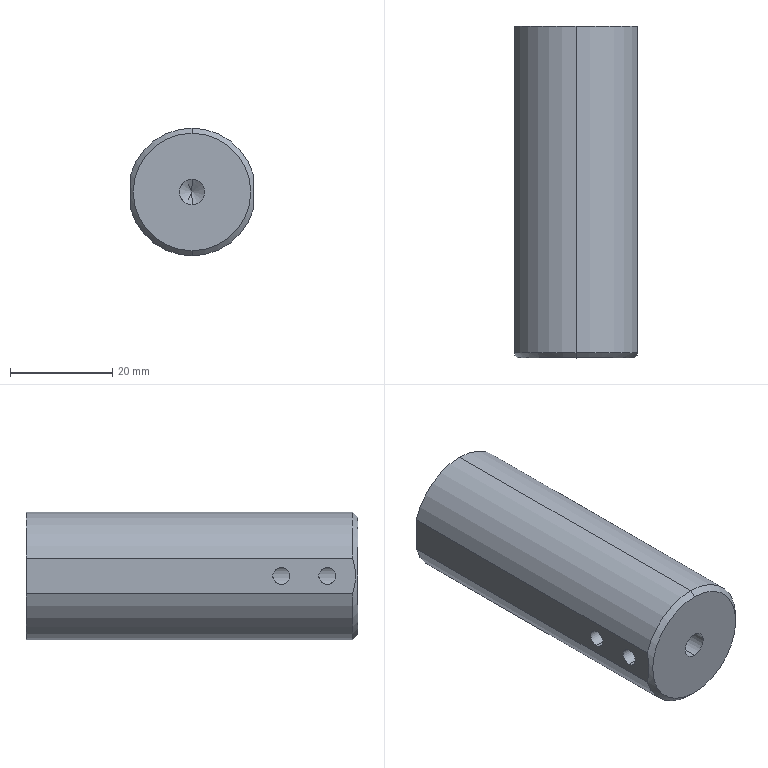Part | SolidWorks | features HoleWzd 3, ICE 2, Chamfer 1, Extrusion 1, MirrorPattern 1 | 1 solid | 27 faces | box 24 x 65 x 25 mm | volume 25326 mm3 | cone 12 | cylinder 11 | plane 4 | commonest cylinder face diameters 3.3 x4 25 x3 5 x2 16.5 x2
STEP:
#1=CARTESIAN_POINT('',(-1.891,-59.,1.635));
#2=VERTEX_POINT('',#1);
#3=CARTESIAN_POINT('',(-1.9,-58.713,1.625));
#4=VERTEX_POINT('',#3);
#5=CARTESIAN_POINT('',(-1.891,-59.,1.635));
#6=CARTESIAN_POINT('',(-1.891,-58.904,1.635));
#7=CARTESIAN_POINT('',(-1.894,-58.808,1.632));
#8=CARTESIAN_POINT('',(-1.9,-58.713,1.625));
#9=B_SPLINE_CURVE_WITH_KNOTS('',3,(#5,#6,#7,#8),.UNSPECIFIED.,.F.,.F.,(4,4),(0.001036,0.001322),.UNSPECIFIED.);
#10=EDGE_CURVE('',#2,#4,#9,.T.);
#11=ORIENTED_EDGE('',*,*,#10,.F.);
#12=CARTESIAN_POINT('',(-1.9,-59.,1.65));
#13=VERTEX_POINT('',#12);
#14=CARTESIAN_POINT('',(-1.9,-59.,1.65));
#15=DIRECTION('',(-0.515,0.,0.8572));
#16=VECTOR('',#15,1000.);
#17=LINE('',#14,#16);
#18=EDGE_CURVE('',#2,#13,#17,.T.);
#19=ORIENTED_EDGE('',*,*,#18,.T.);
#20=CARTESIAN_POINT('',(-1.9,-59.,0.));
#21=DIRECTION('',(-1.,0.,0.));
#22=DIRECTION('',(0.,0.,1.));
#23=AXIS2_PLACEMENT_3D('',#20,#21,#22);
#24=CIRCLE('',#23,1.65);
#25=EDGE_CURVE('',#13,#4,#24,.T.);
#26=ORIENTED_EDGE('',*,*,#25,.T.);
#27=EDGE_LOOP('',(#11,#19,#26));
#28=FACE_OUTER_BOUND('',#27,.T.);
#29=CARTESIAN_POINT('',(-1.9,-59.,0.));
#30=DIRECTION('',(-1.,0.,0.));
#31=DIRECTION('',(0.,0.,1.));
#32=AXIS2_PLACEMENT_3D('',#29,#30,#31);
#33=CONICAL_SURFACE('',#32,1.65,1.03);
#34=ADVANCED_FACE('',(#28),#33,.F.);
#35=CARTESIAN_POINT('',(-1.9,-59.,-1.65));
#36=VERTEX_POINT('',#35);
#37=CARTESIAN_POINT('',(-1.9,-59.287,-1.625));
#38=VERTEX_POINT('',#37);
#39=CARTESIAN_POINT('',(-1.9,-59.,0.));
#40=DIRECTION('',(-1.,0.,0.));
#41=DIRECTION('',(0.,0.,1.));
#42=AXIS2_PLACEMENT_3D('',#39,#40,#41);
#43=CIRCLE('',#42,1.65);
#44=EDGE_CURVE('',#36,#38,#43,.T.);
#45=ORIENTED_EDGE('',*,*,#44,.F.);
#46=CARTESIAN_POINT('',(-12.,-59.,-1.65));
#47=VERTEX_POINT('',#46);
#48=CARTESIAN_POINT('',(-12.,-59.,-1.65));
#49=DIRECTION('',(-1.,0.,0.));
#50=VECTOR('',#49,1000.);
#51=LINE('',#48,#50);
#52=EDGE_CURVE('',#36,#47,#51,.T.);
#53=ORIENTED_EDGE('',*,*,#52,.T.);
#54=CARTESIAN_POINT('',(-12.,-59.,1.65));
#55=VERTEX_POINT('',#54);
#56=CARTESIAN_POINT('',(-12.,-59.,0.));
#57=DIRECTION('',(-1.,0.,0.));
#58=DIRECTION('',(0.,0.,1.));
#59=AXIS2_PLACEMENT_3D('',#56,#57,#58);
#60=CIRCLE('',#59,1.65);
#61=EDGE_CURVE('',#47,#55,#60,.T.);
#62=ORIENTED_EDGE('',*,*,#61,.T.);
#63=CARTESIAN_POINT('',(-12.,-59.,1.65));
#64=DIRECTION('',(-1.,0.,0.));
#65=VECTOR('',#64,1000.);
#66=LINE('',#63,#65);
#67=EDGE_CURVE('',#13,#55,#66,.T.);
#68=ORIENTED_EDGE('',*,*,#67,.F.);
#69=CARTESIAN_POINT('',(-1.9,-59.287,1.625));
#70=VERTEX_POINT('',#69);
#71=CARTESIAN_POINT('',(-1.9,-59.,0.));
#72=DIRECTION('',(-1.,0.,0.));
#73=DIRECTION('',(0.,0.,1.));
#74=AXIS2_PLACEMENT_3D('',#71,#72,#73);
#75=CIRCLE('',#74,1.65);
#76=EDGE_CURVE('',#70,#13,#75,.T.);
#77=ORIENTED_EDGE('',*,*,#76,.F.);
#78=CARTESIAN_POINT('',(-1.9,-59.287,-1.625));
#79=CARTESIAN_POINT('',(-1.93,-59.484,-1.59));
#80=CARTESIAN_POINT('',(-1.986,-59.663,-1.523));
#81=CARTESIAN_POINT('',(-2.118,-59.99,-1.333));
#82=CARTESIAN_POINT('',(-2.192,-60.134,-1.213));
#83=CARTESIAN_POINT('',(-2.327,-60.377,-0.9282));
#84=CARTESIAN_POINT('',(-2.388,-60.475,-0.7644));
#85=CARTESIAN_POINT('',(-2.453,-60.578,-0.4906));
#86=CARTESIAN_POINT('',(-2.47,-60.605,-0.3964));
#87=CARTESIAN_POINT('',(-2.494,-60.641,-0.2018));
#88=CARTESIAN_POINT('',(-2.5,-60.65,-0.1009));
#89=CARTESIAN_POINT('',(-2.5,-60.65,0.1969));
#90=CARTESIAN_POINT('',(-2.475,-60.613,0.3967));
#91=CARTESIAN_POINT('',(-2.41,-60.511,0.6696));
#92=CARTESIAN_POINT('',(-2.384,-60.469,0.7576));
#93=CARTESIAN_POINT('',(-2.325,-60.372,0.9219));
#94=CARTESIAN_POINT('',(-2.293,-60.317,0.9984));
#95=CARTESIAN_POINT('',(-2.192,-60.134,1.213));
#96=CARTESIAN_POINT('',(-2.118,-59.991,1.333));
#97=CARTESIAN_POINT('',(-1.986,-59.664,1.522));
#98=CARTESIAN_POINT('',(-1.93,-59.484,1.59));
#99=CARTESIAN_POINT('',(-1.9,-59.287,1.625));
#100=B_SPLINE_CURVE_WITH_KNOTS('',3,(#78,#79,#80,#81,#82,#83,#84,#85,#86,#87,#88,#89,#90,#91,#92,#93,#94,#95,#96,#97,#98,#99),.UNSPECIFIED.,.F.,.F.,(4,2,2,2,2,2,2,2,2,2,4),(0.,0.0005938,0.001188,0.001781,0.002078,0.002375,0.002969,0.003266,0.003563,0.004157,0.00475),.UNSPECIFIED.);
#101=EDGE_CURVE('',#38,#70,#100,.T.);
#102=ORIENTED_EDGE('',*,*,#101,.F.);
#103=EDGE_LOOP('',(#45,#53,#62,#68,#77,#102));
#104=FACE_OUTER_BOUND('',#103,.T.);
#105=CARTESIAN_POINT('',(-12.,-59.,0.));
#106=DIRECTION('',(-1.,0.,0.));
#107=DIRECTION('',(0.,0.,1.));
#108=AXIS2_PLACEMENT_3D('',#105,#106,#107);
#109=CYLINDRICAL_SURFACE('',#108,1.65);
#110=ADVANCED_FACE('',(#104),#109,.F.);
#111=CARTESIAN_POINT('',(-1.9,-50.,-1.65));
#112=VERTEX_POINT('',#111);
#113=CARTESIAN_POINT('',(-1.9,-50.287,-1.625));
#114=VERTEX_POINT('',#113);
#115=CARTESIAN_POINT('',(-1.9,-50.,0.));
#116=DIRECTION('',(-1.,0.,0.));
#117=DIRECTION('',(0.,0.,1.));
#118=AXIS2_PLACEMENT_3D('',#115,#116,#117);
#119=CIRCLE('',#118,1.65);
#120=EDGE_CURVE('',#112,#114,#119,.T.);
#121=ORIENTED_EDGE('',*,*,#120,.F.);
#122=CARTESIAN_POINT('',(-12.,-50.,-1.65));
#123=VERTEX_POINT('',#122);
#124=CARTESIAN_POINT('',(-12.,-50.,-1.65));
#125=DIRECTION('',(-1.,0.,0.));
#126=VECTOR('',#125,1000.);
#127=LINE('',#124,#126);
#128=EDGE_CURVE('',#112,#123,#127,.T.);
#129=ORIENTED_EDGE('',*,*,#128,.T.);
#130=CARTESIAN_POINT('',(-12.,-50.,1.65));
#131=VERTEX_POINT('',#130);
#132=CARTESIAN_POINT('',(-12.,-50.,0.));
#133=DIRECTION('',(-1.,0.,0.));
#134=DIRECTION('',(0.,0.,1.));
#135=AXIS2_PLACEMENT_3D('',#132,#133,#134);
#136=CIRCLE('',#135,1.65);
#137=EDGE_CURVE('',#123,#131,#136,.T.);
#138=ORIENTED_EDGE('',*,*,#137,.T.);
#139=CARTESIAN_POINT('',(-1.9,-50.,1.65));
#140=VERTEX_POINT('',#139);
#141=CARTESIAN_POINT('',(-12.,-50.,1.65));
#142=DIRECTION('',(-1.,0.,0.));
#143=VECTOR('',#142,1000.);
#144=LINE('',#141,#143);
#145=EDGE_CURVE('',#140,#131,#144,.T.);
#146=ORIENTED_EDGE('',*,*,#145,.F.);
#147=CARTESIAN_POINT('',(-1.9,-50.287,1.625));
#148=VERTEX_POINT('',#147);
#149=CARTESIAN_POINT('',(-1.9,-50.,0.));
#150=DIRECTION('',(-1.,0.,0.));
#151=DIRECTION('',(0.,0.,1.));
#152=AXIS2_PLACEMENT_3D('',#149,#150,#151);
#153=CIRCLE('',#152,1.65);
#154=EDGE_CURVE('',#148,#140,#153,.T.);
#155=ORIENTED_EDGE('',*,*,#154,.F.);
#156=CARTESIAN_POINT('',(-1.9,-50.287,-1.625));
#157=CARTESIAN_POINT('',(-1.93,-50.484,-1.59));
#158=CARTESIAN_POINT('',(-1.986,-50.663,-1.523));
#159=CARTESIAN_POINT('',(-2.118,-50.99,-1.333));
#160=CARTESIAN_POINT('',(-2.192,-51.134,-1.213));
#161=CARTESIAN_POINT('',(-2.327,-51.377,-0.9282));
#162=CARTESIAN_POINT('',(-2.388,-51.475,-0.7644));
#163=CARTESIAN_POINT('',(-2.453,-51.578,-0.4906));
#164=CARTESIAN_POINT('',(-2.47,-51.605,-0.3964));
#165=CARTESIAN_POINT('',(-2.494,-51.641,-0.2018));
#166=CARTESIAN_POINT('',(-2.5,-51.65,-0.1009));
#167=CARTESIAN_POINT('',(-2.5,-51.65,0.1969));
#168=CARTESIAN_POINT('',(-2.475,-51.613,0.3967));
#169=CARTESIAN_POINT('',(-2.41,-51.511,0.6696));
#170=CARTESIAN_POINT('',(-2.384,-51.469,0.7576));
#171=CARTESIAN_POINT('',(-2.325,-51.372,0.9219));
#172=CARTESIAN_POINT('',(-2.293,-51.317,0.9984));
#173=CARTESIAN_POINT('',(-2.192,-51.134,1.213));
#174=CARTESIAN_POINT('',(-2.118,-50.991,1.333));
#175=CARTESIAN_POINT('',(-1.986,-50.664,1.522));
#176=CARTESIAN_POINT('',(-1.93,-50.484,1.59));
#177=CARTESIAN_POINT('',(-1.9,-50.287,1.625));
#178=B_SPLINE_CURVE_WITH_KNOTS('',3,(#156,#157,#158,#159,#160,#161,#162,#163,#164,#165,#166,#167,#168,#169,#170,#171,#172,#173,#174,#175,#176,#177),.UNSPECIFIED.,.F.,.F.,(4,2,2,2,2,2,2,2,2,2,4),(0.,0.0005938,0.001188,0.001781,0.002078,0.002375,0.002969,0.003266,0.003563,0.004157,0.00475),.UNSPECIFIED.);
#179=EDGE_CURVE('',#114,#148,#178,.T.);
#180=ORIENTED_EDGE('',*,*,#179,.F.);
#181=EDGE_LOOP('',(#121,#129,#138,#146,#155,#180));
#182=FACE_OUTER_BOUND('',#181,.T.);
#183=CARTESIAN_POINT('',(-12.,-50.,0.));
#184=DIRECTION('',(-1.,0.,0.));
#185=DIRECTION('',(0.,0.,1.));
#186=AXIS2_PLACEMENT_3D('',#183,#184,#185);
#187=CYLINDRICAL_SURFACE('',#186,1.65);
#188=ADVANCED_FACE('',(#182),#187,.F.);
#189=CARTESIAN_POINT('',(-1.891,-50.,1.635));
#190=VERTEX_POINT('',#189);
#191=CARTESIAN_POINT('',(-1.9,-49.713,1.625));
#192=VERTEX_POINT('',#191);
#193=CARTESIAN_POINT('',(-1.891,-50.,1.635));
#194=CARTESIAN_POINT('',(-1.891,-49.904,1.635));
#195=CARTESIAN_POINT('',(-1.894,-49.808,1.632));
#196=CARTESIAN_POINT('',(-1.9,-49.713,1.625));
#197=B_SPLINE_CURVE_WITH_KNOTS('',3,(#193,#194,#195,#196),.UNSPECIFIED.,.F.,.F.,(4,4),(0.001036,0.001322),.UNSPECIFIED.);
#198=EDGE_CURVE('',#190,#192,#197,.T.);
#199=ORIENTED_EDGE('',*,*,#198,.F.);
#200=CARTESIAN_POINT('',(-1.9,-50.,1.65));
#201=DIRECTION('',(-0.515,0.,0.8572));
#202=VECTOR('',#201,1000.);
#203=LINE('',#200,#202);
#204=EDGE_CURVE('',#190,#140,#203,.T.);
#205=ORIENTED_EDGE('',*,*,#204,.T.);
#206=CARTESIAN_POINT('',(-1.9,-50.,0.));
#207=DIRECTION('',(-1.,0.,0.));
#208=DIRECTION('',(0.,0.,1.));
#209=AXIS2_PLACEMENT_3D('',#206,#207,#208);
#210=CIRCLE('',#209,1.65);
#211=EDGE_CURVE('',#140,#192,#210,.T.);
#212=ORIENTED_EDGE('',*,*,#211,.T.);
#213=EDGE_LOOP('',(#199,#205,#212));
#214=FACE_OUTER_BOUND('',#213,.T.);
#215=CARTESIAN_POINT('',(-1.9,-50.,0.));
#216=DIRECTION('',(-1.,0.,0.));
#217=DIRECTION('',(0.,0.,1.));
#218=AXIS2_PLACEMENT_3D('',#215,#216,#217);
#219=CONICAL_SURFACE('',#218,1.65,1.03);
#220=ADVANCED_FACE('',(#214),#219,.F.);
#221=CARTESIAN_POINT('',(0.,-65.,-11.5));
#222=VERTEX_POINT('',#221);
#223=CARTESIAN_POINT('',(0.,-65.,11.5));
#224=VERTEX_POINT('',#223);
#225=CARTESIAN_POINT('',(0.,-65.,0.));
#226=DIRECTION('',(0.,-1.,0.));
#227=DIRECTION('',(0.,0.,-1.));
#228=AXIS2_PLACEMENT_3D('',#225,#226,#227);
#229=CIRCLE('',#228,11.5);
#230=EDGE_CURVE('',#222,#224,#229,.T.);
#231=ORIENTED_EDGE('',*,*,#230,.F.);
#232=CARTESIAN_POINT('',(0.,-64.,-12.5));
#233=VERTEX_POINT('',#232);
#234=CARTESIAN_POINT('',(0.,-65.,-11.5));
#235=DIRECTION('',(0.,0.7071,-0.7071));
#236=VECTOR('',#235,1000.);
#237=LINE('',#234,#236);
#238=EDGE_CURVE('',#222,#233,#237,.T.);
#239=ORIENTED_EDGE('',*,*,#238,.T.);
#240=CARTESIAN_POINT('',(12.,-64.,-3.5));
#241=VERTEX_POINT('',#240);
#242=CARTESIAN_POINT('',(0.,-64.,0.));
#243=DIRECTION('',(0.,1.,0.));
#244=DIRECTION('',(0.,0.,-1.));
#245=AXIS2_PLACEMENT_3D('',#242,#243,#244);
#246=CIRCLE('',#245,12.5);
#247=EDGE_CURVE('',#241,#233,#246,.T.);
#248=ORIENTED_EDGE('',*,*,#247,.F.);
#249=CARTESIAN_POINT('',(12.,-64.,3.5));
#250=VERTEX_POINT('',#249);
#251=CARTESIAN_POINT('',(12.,-64.,3.5));
#252=CARTESIAN_POINT('',(12.,-64.321,2.353));
#253=CARTESIAN_POINT('',(12.,-64.5,1.186));
#254=CARTESIAN_POINT('',(12.,-64.5,-0.6002));
#255=CARTESIAN_POINT('',(12.,-64.455,-1.192));
#256=CARTESIAN_POINT('',(12.,-64.284,-2.357));
#257=CARTESIAN_POINT('',(12.,-64.159,-2.931));
#258=CARTESIAN_POINT('',(12.,-64.,-3.5));
#259=B_SPLINE_CURVE_WITH_KNOTS('',3,(#251,#252,#253,#254,#255,#256,#257,#258),.UNSPECIFIED.,.F.,.F.,(4,2,2,4),(0.,0.00354,0.00531,0.00708),.UNSPECIFIED.);
#260=EDGE_CURVE('',#250,#241,#259,.T.);
#261=ORIENTED_EDGE('',*,*,#260,.F.);
#262=CARTESIAN_POINT('',(0.,-64.,12.5));
#263=VERTEX_POINT('',#262);
#264=CARTESIAN_POINT('',(0.,-64.,0.));
#265=DIRECTION('',(0.,1.,0.));
#266=DIRECTION('',(0.,0.,1.));
#267=AXIS2_PLACEMENT_3D('',#264,#265,#266);
#268=CIRCLE('',#267,12.5);
#269=EDGE_CURVE('',#263,#250,#268,.T.);
#270=ORIENTED_EDGE('',*,*,#269,.F.);
#271=CARTESIAN_POINT('',(0.,-65.,11.5));
#272=DIRECTION('',(0.,0.7071,0.7071));
#273=VECTOR('',#272,1000.);
#274=LINE('',#271,#273);
#275=EDGE_CURVE('',#224,#263,#274,.T.);
#276=ORIENTED_EDGE('',*,*,#275,.F.);
#277=EDGE_LOOP('',(#231,#239,#248,#261,#270,#276));
#278=FACE_OUTER_BOUND('',#277,.T.);
#279=CARTESIAN_POINT('',(0.,-65.,0.));
#280=DIRECTION('',(0.,1.,0.));
#281=DIRECTION('',(0.,0.,1.));
#282=AXIS2_PLACEMENT_3D('',#279,#280,#281);
#283=CONICAL_SURFACE('',#282,11.5,0.7854);
#284=ADVANCED_FACE('',(#278),#283,.T.);
#285=ORIENTED_EDGE('',*,*,#101,.T.);
#286=CARTESIAN_POINT('',(-1.9,-59.287,1.625));
#287=CARTESIAN_POINT('',(-1.894,-59.192,1.632));
#288=CARTESIAN_POINT('',(-1.891,-59.096,1.635));
#289=CARTESIAN_POINT('',(-1.891,-59.,1.635));
#290=B_SPLINE_CURVE_WITH_KNOTS('',3,(#286,#287,#288,#289),.UNSPECIFIED.,.F.,.F.,(4,4),(0.0007504,0.001036),.UNSPECIFIED.);
#291=EDGE_CURVE('',#70,#2,#290,.T.);
#292=ORIENTED_EDGE('',*,*,#291,.T.);
#293=ORIENTED_EDGE('',*,*,#10,.T.);
#294=CARTESIAN_POINT('',(-1.9,-58.713,-1.625));
#295=VERTEX_POINT('',#294);
#296=CARTESIAN_POINT('',(-1.9,-58.713,1.625));
#297=CARTESIAN_POINT('',(-1.93,-58.516,1.59));
#298=CARTESIAN_POINT('',(-1.986,-58.337,1.523));
#299=CARTESIAN_POINT('',(-2.118,-58.01,1.333));
#300=CARTESIAN_POINT('',(-2.192,-57.866,1.213));
#301=CARTESIAN_POINT('',(-2.327,-57.623,0.9282));
#302=CARTESIAN_POINT('',(-2.388,-57.525,0.7644));
#303=CARTESIAN_POINT('',(-2.453,-57.422,0.4906));
#304=CARTESIAN_POINT('',(-2.47,-57.395,0.3964));
#305=CARTESIAN_POINT('',(-2.494,-57.359,0.2018));
#306=CARTESIAN_POINT('',(-2.5,-57.35,0.1009));
#307=CARTESIAN_POINT('',(-2.5,-57.35,-0.1969));
#308=CARTESIAN_POINT('',(-2.475,-57.387,-0.3967));
#309=CARTESIAN_POINT('',(-2.41,-57.489,-0.6696));
#310=CARTESIAN_POINT('',(-2.384,-57.531,-0.7576));
#311=CARTESIAN_POINT('',(-2.325,-57.628,-0.9219));
#312=CARTESIAN_POINT('',(-2.293,-57.683,-0.9984));
#313=CARTESIAN_POINT('',(-2.192,-57.866,-1.213));
#314=CARTESIAN_POINT('',(-2.118,-58.009,-1.333));
#315=CARTESIAN_POINT('',(-1.986,-58.336,-1.522));
#316=CARTESIAN_POINT('',(-1.93,-58.516,-1.59));
#317=CARTESIAN_POINT('',(-1.9,-58.713,-1.625));
#318=B_SPLINE_CURVE_WITH_KNOTS('',3,(#296,#297,#298,#299,#300,#301,#302,#303,#304,#305,#306,#307,#308,#309,#310,#311,#312,#313,#314,#315,#316,#317),.UNSPECIFIED.,.F.,.F.,(4,2,2,2,2,2,2,2,2,2,4),(0.,0.0005938,0.001188,0.001781,0.002078,0.002375,0.002969,0.003266,0.003563,0.004157,0.00475),.UNSPECIFIED.);
#319=EDGE_CURVE('',#4,#295,#318,.T.);
#320=ORIENTED_EDGE('',*,*,#319,.T.);
#321=CARTESIAN_POINT('',(-1.9,-58.713,-1.625));
#322=CARTESIAN_POINT('',(-1.888,-58.903,-1.639));
#323=CARTESIAN_POINT('',(-1.888,-59.098,-1.639));
#324=CARTESIAN_POINT('',(-1.9,-59.287,-1.625));
#325=B_SPLINE_CURVE_WITH_KNOTS('',3,(#321,#322,#323,#324),.UNSPECIFIED.,.F.,.F.,(4,4),(0.0007504,0.001322),.UNSPECIFIED.);
#326=EDGE_CURVE('',#295,#38,#325,.T.);
#327=ORIENTED_EDGE('',*,*,#326,.T.);
#328=EDGE_LOOP('',(#285,#292,#293,#320,#327));
#329=FACE_BOUND('',#328,.T.);
#330=CARTESIAN_POINT('',(-1.9,-49.713,-1.625));
#331=VERTEX_POINT('',#330);
#332=CARTESIAN_POINT('',(-1.9,-49.713,-1.625));
#333=CARTESIAN_POINT('',(-1.888,-49.903,-1.639));
#334=CARTESIAN_POINT('',(-1.888,-50.098,-1.639));
#335=CARTESIAN_POINT('',(-1.9,-50.287,-1.625));
#336=B_SPLINE_CURVE_WITH_KNOTS('',3,(#332,#333,#334,#335),.UNSPECIFIED.,.F.,.F.,(4,4),(0.0007504,0.001322),.UNSPECIFIED.);
#337=EDGE_CURVE('',#331,#114,#336,.T.);
#338=ORIENTED_EDGE('',*,*,#337,.T.);
#339=ORIENTED_EDGE('',*,*,#179,.T.);
#340=CARTESIAN_POINT('',(-1.9,-50.287,1.625));
#341=CARTESIAN_POINT('',(-1.894,-50.192,1.632));
#342=CARTESIAN_POINT('',(-1.891,-50.096,1.635));
#343=CARTESIAN_POINT('',(-1.891,-50.,1.635));
#344=B_SPLINE_CURVE_WITH_KNOTS('',3,(#340,#341,#342,#343),.UNSPECIFIED.,.F.,.F.,(4,4),(0.0007504,0.001036),.UNSPECIFIED.);
#345=EDGE_CURVE('',#148,#190,#344,.T.);
#346=ORIENTED_EDGE('',*,*,#345,.T.);
#347=ORIENTED_EDGE('',*,*,#198,.T.);
#348=CARTESIAN_POINT('',(-1.9,-49.713,1.625));
#349=CARTESIAN_POINT('',(-1.93,-49.516,1.59));
#350=CARTESIAN_POINT('',(-1.986,-49.337,1.523));
#351=CARTESIAN_POINT('',(-2.118,-49.01,1.333));
#352=CARTESIAN_POINT('',(-2.192,-48.866,1.213));
#353=CARTESIAN_POINT('',(-2.327,-48.623,0.9282));
#354=CARTESIAN_POINT('',(-2.388,-48.525,0.7644));
#355=CARTESIAN_POINT('',(-2.453,-48.422,0.4906));
#356=CARTESIAN_POINT('',(-2.47,-48.395,0.3964));
#357=CARTESIAN_POINT('',(-2.494,-48.359,0.2018));
#358=CARTESIAN_POINT('',(-2.5,-48.35,0.1009));
#359=CARTESIAN_POINT('',(-2.5,-48.35,-0.1969));
#360=CARTESIAN_POINT('',(-2.475,-48.387,-0.3967));
#361=CARTESIAN_POINT('',(-2.41,-48.489,-0.6696));
#362=CARTESIAN_POINT('',(-2.384,-48.531,-0.7576));
#363=CARTESIAN_POINT('',(-2.325,-48.628,-0.9219));
#364=CARTESIAN_POINT('',(-2.293,-48.683,-0.9984));
#365=CARTESIAN_POINT('',(-2.192,-48.866,-1.213));
#366=CARTESIAN_POINT('',(-2.118,-49.009,-1.333));
#367=CARTESIAN_POINT('',(-1.986,-49.336,-1.522));
#368=CARTESIAN_POINT('',(-1.93,-49.516,-1.59));
#369=CARTESIAN_POINT('',(-1.9,-49.713,-1.625));
#370=B_SPLINE_CURVE_WITH_KNOTS('',3,(#348,#349,#350,#351,#352,#353,#354,#355,#356,#357,#358,#359,#360,#361,#362,#363,#364,#365,#366,#367,#368,#369),.UNSPECIFIED.,.F.,.F.,(4,2,2,2,2,2,2,2,2,2,4),(0.,0.0005938,0.001188,0.001781,0.002078,0.002375,0.002969,0.003266,0.003563,0.004157,0.00475),.UNSPECIFIED.);
#371=EDGE_CURVE('',#192,#331,#370,.T.);
#372=ORIENTED_EDGE('',*,*,#371,.T.);
#373=EDGE_LOOP('',(#338,#339,#346,#347,#372));
#374=FACE_BOUND('',#373,.T.);
#375=CARTESIAN_POINT('',(0.,-46.25,2.5));
#376=VERTEX_POINT('',#375);
#377=CARTESIAN_POINT('',(0.,-46.25,-2.5));
#378=VERTEX_POINT('',#377);
#379=CARTESIAN_POINT('',(0.,-46.25,0.));
#380=DIRECTION('',(0.,-1.,0.));
#381=DIRECTION('',(0.,0.,-1.));
#382=AXIS2_PLACEMENT_3D('',#379,#380,#381);
#383=CIRCLE('',#382,2.5);
#384=EDGE_CURVE('',#376,#378,#383,.T.);
#385=ORIENTED_EDGE('',*,*,#384,.F.);
#386=CARTESIAN_POINT('',(0.,-65.,2.5));
#387=VERTEX_POINT('',#386);
#388=CARTESIAN_POINT('',(0.,-65.,2.5));
#389=DIRECTION('',(0.,-1.,0.));
#390=VECTOR('',#389,1000.);
#391=LINE('',#388,#390);
#392=EDGE_CURVE('',#376,#387,#391,.T.);
#393=ORIENTED_EDGE('',*,*,#392,.T.);
#394=CARTESIAN_POINT('',(0.,-65.,-2.5));
#395=VERTEX_POINT('',#394);
#396=CARTESIAN_POINT('',(0.,-65.,0.));
#397=DIRECTION('',(0.,-1.,0.));
#398=DIRECTION('',(0.,0.,-1.));
#399=AXIS2_PLACEMENT_3D('',#396,#397,#398);
#400=CIRCLE('',#399,2.5);
#401=EDGE_CURVE('',#387,#395,#400,.T.);
#402=ORIENTED_EDGE('',*,*,#401,.T.);
#403=CARTESIAN_POINT('',(0.,-65.,-2.5));
#404=DIRECTION('',(0.,-1.,0.));
#405=VECTOR('',#404,1000.);
#406=LINE('',#403,#405);
#407=EDGE_CURVE('',#378,#395,#406,.T.);
#408=ORIENTED_EDGE('',*,*,#407,.F.);
#409=EDGE_LOOP('',(#385,#393,#402,#408));
#410=FACE_OUTER_BOUND('',#409,.T.);
#411=CARTESIAN_POINT('',(0.,-65.,0.));
#412=DIRECTION('',(0.,-1.,0.));
#413=DIRECTION('',(0.,0.,-1.));
#414=AXIS2_PLACEMENT_3D('',#411,#412,#413);
#415=CYLINDRICAL_SURFACE('',#414,2.5);
#416=ADVANCED_FACE('',(#329,#374,#410),#415,.F.);
#417=CARTESIAN_POINT('',(0.,-44.748,0.));
#418=VERTEX_POINT('',#417);
#419=CARTESIAN_POINT('',(0.,-46.25,-2.5));
#420=DIRECTION('',(0.,-0.515,-0.8572));
#421=VECTOR('',#420,1000.);
#422=LINE('',#419,#421);
#423=EDGE_CURVE('',#418,#378,#422,.T.);
#424=ORIENTED_EDGE('',*,*,#423,.F.);
#425=CARTESIAN_POINT('',(0.,-46.25,2.5));
#426=DIRECTION('',(0.,-0.515,0.8572));
#427=VECTOR('',#426,1000.);
#428=LINE('',#425,#427);
#429=EDGE_CURVE('',#418,#376,#428,.T.);
#430=ORIENTED_EDGE('',*,*,#429,.T.);
#431=ORIENTED_EDGE('',*,*,#384,.T.);
#432=EDGE_LOOP('',(#424,#430,#431));
#433=FACE_OUTER_BOUND('',#432,.T.);
#434=CARTESIAN_POINT('',(0.,-46.25,0.));
#435=DIRECTION('',(0.,-1.,0.));
#436=DIRECTION('',(0.,0.,-1.));
#437=AXIS2_PLACEMENT_3D('',#434,#435,#436);
#438=CONICAL_SURFACE('',#437,2.5,1.03);
#439=ADVANCED_FACE('',(#433),#438,.F.);
#440=CARTESIAN_POINT('',(0.,-25.,-8.25));
#441=VERTEX_POINT('',#440);
#442=CARTESIAN_POINT('',(0.,-25.,8.25));
#443=VERTEX_POINT('',#442);
#444=CARTESIAN_POINT('',(0.,-25.,0.));
#445=DIRECTION('',(0.,1.,0.));
#446=DIRECTION('',(0.,0.,1.));
#447=AXIS2_PLACEMENT_3D('',#444,#445,#446);
#448=CIRCLE('',#447,8.25);
#449=EDGE_CURVE('',#441,#443,#448,.T.);
#450=ORIENTED_EDGE('',*,*,#449,.F.);
#451=CARTESIAN_POINT('',(0.,0.,-8.25));
#452=VERTEX_POINT('',#451);
#453=CARTESIAN_POINT('',(0.,0.,-8.25));
#454=DIRECTION('',(0.,1.,0.));
#455=VECTOR('',#454,1000.);
#456=LINE('',#453,#455);
#457=EDGE_CURVE('',#441,#452,#456,.T.);
#458=ORIENTED_EDGE('',*,*,#457,.T.);
#459=CARTESIAN_POINT('',(0.,0.,8.25));
#460=VERTEX_POINT('',#459);
#461=CARTESIAN_POINT('',(0.,0.,0.));
#462=DIRECTION('',(0.,1.,0.));
#463=DIRECTION('',(0.,0.,1.));
#464=AXIS2_PLACEMENT_3D('',#461,#462,#463);
#465=CIRCLE('',#464,8.25);
#466=EDGE_CURVE('',#452,#460,#465,.T.);
#467=ORIENTED_EDGE('',*,*,#466,.T.);
#468=CARTESIAN_POINT('',(0.,0.,8.25));
#469=DIRECTION('',(0.,1.,0.));
#470=VECTOR('',#469,1000.);
#471=LINE('',#468,#470);
#472=EDGE_CURVE('',#443,#460,#471,.T.);
#473=ORIENTED_EDGE('',*,*,#472,.F.);
#474=EDGE_LOOP('',(#450,#458,#467,#473));
#475=FACE_OUTER_BOUND('',#474,.T.);
#476=CARTESIAN_POINT('',(0.,0.,0.));
#477=DIRECTION('',(0.,1.,0.));
#478=DIRECTION('',(0.,0.,1.));
#479=AXIS2_PLACEMENT_3D('',#476,#477,#478);
#480=CYLINDRICAL_SURFACE('',#479,8.25);
#481=ADVANCED_FACE('',(#475),#480,.F.);
#482=CARTESIAN_POINT('',(0.,-29.957,0.));
#483=VERTEX_POINT('',#482);
#484=CARTESIAN_POINT('',(0.,-25.,8.25));
#485=DIRECTION('',(0.,0.515,0.8572));
#486=VECTOR('',#485,1000.);
#487=LINE('',#484,#486);
#488=EDGE_CURVE('',#483,#443,#487,.T.);
#489=ORIENTED_EDGE('',*,*,#488,.F.);
#490=CARTESIAN_POINT('',(0.,-25.,-8.25));
#491=DIRECTION('',(0.,0.515,-0.8572));
#492=VECTOR('',#491,1000.);
#493=LINE('',#490,#492);
#494=EDGE_CURVE('',#483,#441,#493,.T.);
#495=ORIENTED_EDGE('',*,*,#494,.T.);
#496=ORIENTED_EDGE('',*,*,#449,.T.);
#497=EDGE_LOOP('',(#489,#495,#496));
#498=FACE_OUTER_BOUND('',#497,.T.);
#499=CARTESIAN_POINT('',(0.,-25.,0.));
#500=DIRECTION('',(0.,1.,0.));
#501=DIRECTION('',(0.,0.,1.));
#502=AXIS2_PLACEMENT_3D('',#499,#500,#501);
#503=CONICAL_SURFACE('',#502,8.25,1.03);
#504=ADVANCED_FACE('',(#498),#503,.F.);
#505=CARTESIAN_POINT('',(-12.,-64.,3.5));
#506=VERTEX_POINT('',#505);
#507=CARTESIAN_POINT('',(0.,-64.,0.));
#508=DIRECTION('',(0.,1.,0.));
#509=DIRECTION('',(0.,0.,1.));
#510=AXIS2_PLACEMENT_3D('',#507,#508,#509);
#511=CIRCLE('',#510,12.5);
#512=EDGE_CURVE('',#506,#263,#511,.T.);
#513=ORIENTED_EDGE('',*,*,#512,.T.);
#514=CARTESIAN_POINT('',(0.,0.,12.5));
#515=VERTEX_POINT('',#514);
#516=CARTESIAN_POINT('',(0.,-30.,12.5));
#517=DIRECTION('',(0.,1.,0.));
#518=VECTOR('',#517,1000.);
#519=LINE('',#516,#518);
#520=EDGE_CURVE('',#263,#515,#519,.T.);
#521=ORIENTED_EDGE('',*,*,#520,.T.);
#522=CARTESIAN_POINT('',(-12.,0.,3.5));
#523=VERTEX_POINT('',#522);
#524=CARTESIAN_POINT('',(0.,0.,0.));
#525=DIRECTION('',(0.,1.,0.));
#526=DIRECTION('',(0.,0.,1.));
#527=AXIS2_PLACEMENT_3D('',#524,#525,#526);
#528=CIRCLE('',#527,12.5);
#529=EDGE_CURVE('',#523,#515,#528,.T.);
#530=ORIENTED_EDGE('',*,*,#529,.F.);
#531=CARTESIAN_POINT('',(-12.,-30.,3.5));
#532=DIRECTION('',(0.,1.,0.));
#533=VECTOR('',#532,1000.);
#534=LINE('',#531,#533);
#535=EDGE_CURVE('',#506,#523,#534,.T.);
#536=ORIENTED_EDGE('',*,*,#535,.F.);
#537=EDGE_LOOP('',(#513,#521,#530,#536));
#538=FACE_OUTER_BOUND('',#537,.T.);
#539=CARTESIAN_POINT('',(0.,-30.,0.));
#540=DIRECTION('',(0.,1.,0.));
#541=DIRECTION('',(0.,0.,1.));
#542=AXIS2_PLACEMENT_3D('',#539,#540,#541);
#543=CYLINDRICAL_SURFACE('',#542,12.5);
#544=ADVANCED_FACE('',(#538),#543,.T.);
#545=CARTESIAN_POINT('',(12.,0.,-3.5));
#546=VERTEX_POINT('',#545);
#547=CARTESIAN_POINT('',(12.,-30.,-3.5));
#548=DIRECTION('',(0.,-1.,0.));
#549=VECTOR('',#548,1000.);
#550=LINE('',#547,#549);
#551=EDGE_CURVE('',#546,#241,#550,.T.);
#552=ORIENTED_EDGE('',*,*,#551,.T.);
#553=ORIENTED_EDGE('',*,*,#247,.T.);
#554=CARTESIAN_POINT('',(-12.,-64.,-3.5));
#555=VERTEX_POINT('',#554);
#556=CARTESIAN_POINT('',(0.,-64.,0.));
#557=DIRECTION('',(0.,1.,0.));
#558=DIRECTION('',(0.,0.,-1.));
#559=AXIS2_PLACEMENT_3D('',#556,#557,#558);
#560=CIRCLE('',#559,12.5);
#561=EDGE_CURVE('',#233,#555,#560,.T.);
#562=ORIENTED_EDGE('',*,*,#561,.T.);
#563=CARTESIAN_POINT('',(-12.,0.,-3.5));
#564=VERTEX_POINT('',#563);
#565=CARTESIAN_POINT('',(-12.,-30.,-3.5));
#566=DIRECTION('',(0.,-1.,0.));
#567=VECTOR('',#566,1000.);
#568=LINE('',#565,#567);
#569=EDGE_CURVE('',#564,#555,#568,.T.);
#570=ORIENTED_EDGE('',*,*,#569,.F.);
#571=CARTESIAN_POINT('',(0.,0.,0.));
#572=DIRECTION('',(0.,1.,0.));
#573=DIRECTION('',(0.,0.,1.));
#574=AXIS2_PLACEMENT_3D('',#571,#572,#573);
#575=CIRCLE('',#574,12.5);
#576=EDGE_CURVE('',#546,#564,#575,.T.);
#577=ORIENTED_EDGE('',*,*,#576,.F.);
#578=EDGE_LOOP('',(#552,#553,#562,#570,#577));
#579=FACE_OUTER_BOUND('',#578,.T.);
#580=CARTESIAN_POINT('',(0.,-30.,0.));
#581=DIRECTION('',(0.,1.,0.));
#582=DIRECTION('',(0.,0.,1.));
#583=AXIS2_PLACEMENT_3D('',#580,#581,#582);
#584=CYLINDRICAL_SURFACE('',#583,12.5);
#585=ADVANCED_FACE('',(#579),#584,.T.);
#586=ORIENTED_EDGE('',*,*,#520,.F.);
#587=ORIENTED_EDGE('',*,*,#269,.T.);
#588=CARTESIAN_POINT('',(12.,0.,3.5));
#589=VERTEX_POINT('',#588);
#590=CARTESIAN_POINT('',(12.,-30.,3.5));
#591=DIRECTION('',(0.,1.,0.));
#592=VECTOR('',#591,1000.);
#593=LINE('',#590,#592);
#594=EDGE_CURVE('',#250,#589,#593,.T.);
#595=ORIENTED_EDGE('',*,*,#594,.T.);
#596=CARTESIAN_POINT('',(0.,0.,0.));
#597=DIRECTION('',(0.,1.,0.));
#598=DIRECTION('',(0.,0.,1.));
#599=AXIS2_PLACEMENT_3D('',#596,#597,#598);
#600=CIRCLE('',#599,12.5);
#601=EDGE_CURVE('',#515,#589,#600,.T.);
#602=ORIENTED_EDGE('',*,*,#601,.F.);
#603=EDGE_LOOP('',(#586,#587,#595,#602));
#604=FACE_OUTER_BOUND('',#603,.T.);
#605=CARTESIAN_POINT('',(0.,-30.,0.));
#606=DIRECTION('',(0.,1.,0.));
#607=DIRECTION('',(0.,0.,1.));
#608=AXIS2_PLACEMENT_3D('',#605,#606,#607);
#609=CYLINDRICAL_SURFACE('',#608,12.5);
#610=ADVANCED_FACE('',(#604),#609,.T.);
#611=CARTESIAN_POINT('',(0.,0.,0.));
#612=DIRECTION('',(0.,1.,0.));
#613=DIRECTION('',(0.,0.,1.));
#614=AXIS2_PLACEMENT_3D('',#611,#612,#613);
#615=CIRCLE('',#614,8.25);
#616=EDGE_CURVE('',#460,#452,#615,.T.);
#617=ORIENTED_EDGE('',*,*,#616,.F.);
#618=ORIENTED_EDGE('',*,*,#466,.F.);
#619=EDGE_LOOP('',(#617,#618));
#620=FACE_BOUND('',#619,.T.);
#621=ORIENTED_EDGE('',*,*,#529,.T.);
#622=ORIENTED_EDGE('',*,*,#601,.T.);
#623=CARTESIAN_POINT('',(12.,0.,0.));
#624=DIRECTION('',(0.,0.,-1.));
#625=VECTOR('',#624,1000.);
#626=LINE('',#623,#625);
#627=EDGE_CURVE('',#589,#546,#626,.T.);
#628=ORIENTED_EDGE('',*,*,#627,.T.);
#629=ORIENTED_EDGE('',*,*,#576,.T.);
#630=CARTESIAN_POINT('',(-12.,0.,0.));
#631=DIRECTION('',(0.,0.,-1.));
#632=VECTOR('',#631,1000.);
#633=LINE('',#630,#632);
#634=EDGE_CURVE('',#523,#564,#633,.T.);
#635=ORIENTED_EDGE('',*,*,#634,.F.);
#636=EDGE_LOOP('',(#621,#622,#628,#629,#635));
#637=FACE_OUTER_BOUND('',#636,.T.);
#638=CARTESIAN_POINT('',(0.,0.,0.));
#639=DIRECTION('',(0.,1.,0.));
#640=DIRECTION('',(0.,0.,1.));
#641=AXIS2_PLACEMENT_3D('',#638,#639,#640);
#642=PLANE('',#641);
#643=ADVANCED_FACE('',(#620,#637),#642,.T.);
#644=CARTESIAN_POINT('',(0.,-65.,0.));
#645=DIRECTION('',(0.,-1.,0.));
#646=DIRECTION('',(0.,0.,-1.));
#647=AXIS2_PLACEMENT_3D('',#644,#645,#646);
#648=CIRCLE('',#647,11.5);
#649=EDGE_CURVE('',#224,#222,#648,.T.);
#650=ORIENTED_EDGE('',*,*,#649,.T.);
#651=ORIENTED_EDGE('',*,*,#230,.T.);
#652=EDGE_LOOP('',(#650,#651));
#653=FACE_OUTER_BOUND('',#652,.T.);
#654=CARTESIAN_POINT('',(0.,-65.,0.));
#655=DIRECTION('',(0.,-1.,0.));
#656=DIRECTION('',(0.,0.,-1.));
#657=AXIS2_PLACEMENT_3D('',#654,#655,#656);
#658=CIRCLE('',#657,2.5);
#659=EDGE_CURVE('',#395,#387,#658,.T.);
#660=ORIENTED_EDGE('',*,*,#659,.F.);
#661=ORIENTED_EDGE('',*,*,#401,.F.);
#662=EDGE_LOOP('',(#660,#661));
#663=FACE_BOUND('',#662,.T.);
#664=CARTESIAN_POINT('',(0.,-65.,0.));
#665=DIRECTION('',(0.,-1.,0.));
#666=DIRECTION('',(0.,0.,-1.));
#667=AXIS2_PLACEMENT_3D('',#664,#665,#666);
#668=PLANE('',#667);
#669=ADVANCED_FACE('',(#653,#663),#668,.T.);
#670=ORIENTED_EDGE('',*,*,#494,.F.);
#671=ORIENTED_EDGE('',*,*,#488,.T.);
#672=CARTESIAN_POINT('',(0.,-25.,0.));
#673=DIRECTION('',(0.,1.,0.));
#674=DIRECTION('',(0.,0.,1.));
#675=AXIS2_PLACEMENT_3D('',#672,#673,#674);
#676=CIRCLE('',#675,8.25);
#677=EDGE_CURVE('',#443,#441,#676,.T.);
#678=ORIENTED_EDGE('',*,*,#677,.T.);
#679=EDGE_LOOP('',(#670,#671,#678));
#680=FACE_OUTER_BOUND('',#679,.T.);
#681=CARTESIAN_POINT('',(0.,-25.,0.));
#682=DIRECTION('',(0.,1.,0.));
#683=DIRECTION('',(0.,0.,1.));
#684=AXIS2_PLACEMENT_3D('',#681,#682,#683);
#685=CONICAL_SURFACE('',#684,8.25,1.03);
#686=ADVANCED_FACE('',(#680),#685,.F.);
#687=ORIENTED_EDGE('',*,*,#457,.F.);
#688=ORIENTED_EDGE('',*,*,#677,.F.);
#689=ORIENTED_EDGE('',*,*,#472,.T.);
#690=ORIENTED_EDGE('',*,*,#616,.T.);
#691=EDGE_LOOP('',(#687,#688,#689,#690));
#692=FACE_OUTER_BOUND('',#691,.T.);
#693=CARTESIAN_POINT('',(0.,0.,0.));
#694=DIRECTION('',(0.,1.,0.));
#695=DIRECTION('',(0.,0.,1.));
#696=AXIS2_PLACEMENT_3D('',#693,#694,#695);
#697=CYLINDRICAL_SURFACE('',#696,8.25);
#698=ADVANCED_FACE('',(#692),#697,.F.);
#699=CARTESIAN_POINT('',(-12.,-59.,0.));
#700=DIRECTION('',(-1.,0.,0.));
#701=DIRECTION('',(0.,0.,1.));
#702=AXIS2_PLACEMENT_3D('',#699,#700,#701);
#703=CIRCLE('',#702,1.65);
#704=EDGE_CURVE('',#55,#47,#703,.T.);
#705=ORIENTED_EDGE('',*,*,#704,.F.);
#706=ORIENTED_EDGE('',*,*,#61,.F.);
#707=EDGE_LOOP('',(#705,#706));
#708=FACE_BOUND('',#707,.T.);
#709=CARTESIAN_POINT('',(-12.,-50.,0.));
#710=DIRECTION('',(-1.,0.,0.));
#711=DIRECTION('',(0.,0.,1.));
#712=AXIS2_PLACEMENT_3D('',#709,#710,#711);
#713=CIRCLE('',#712,1.65);
#714=EDGE_CURVE('',#131,#123,#713,.T.);
#715=ORIENTED_EDGE('',*,*,#714,.F.);
#716=ORIENTED_EDGE('',*,*,#137,.F.);
#717=EDGE_LOOP('',(#715,#716));
#718=FACE_BOUND('',#717,.T.);
#719=ORIENTED_EDGE('',*,*,#569,.T.);
#720=CARTESIAN_POINT('',(-12.,-64.,-3.5));
#721=CARTESIAN_POINT('',(-12.,-64.321,-2.353));
#722=CARTESIAN_POINT('',(-12.,-64.5,-1.186));
#723=CARTESIAN_POINT('',(-12.,-64.5,0.6002));
#724=CARTESIAN_POINT('',(-12.,-64.455,1.192));
#725=CARTESIAN_POINT('',(-12.,-64.284,2.357));
#726=CARTESIAN_POINT('',(-12.,-64.159,2.931));
#727=CARTESIAN_POINT('',(-12.,-64.,3.5));
#728=B_SPLINE_CURVE_WITH_KNOTS('',3,(#720,#721,#722,#723,#724,#725,#726,#727),.UNSPECIFIED.,.F.,.F.,(4,2,2,4),(0.,0.00354,0.00531,0.00708),.UNSPECIFIED.);
#729=EDGE_CURVE('',#555,#506,#728,.T.);
#730=ORIENTED_EDGE('',*,*,#729,.T.);
#731=ORIENTED_EDGE('',*,*,#535,.T.);
#732=ORIENTED_EDGE('',*,*,#634,.T.);
#733=EDGE_LOOP('',(#719,#730,#731,#732));
#734=FACE_OUTER_BOUND('',#733,.T.);
#735=CARTESIAN_POINT('',(-12.,34.917,-10.));
#736=DIRECTION('',(1.,0.,0.));
#737=DIRECTION('',(0.,0.,-1.));
#738=AXIS2_PLACEMENT_3D('',#735,#736,#737);
#739=PLANE('',#738);
#740=ADVANCED_FACE('',(#708,#718,#734),#739,.F.);
#741=ORIENTED_EDGE('',*,*,#594,.F.);
#742=ORIENTED_EDGE('',*,*,#260,.T.);
#743=ORIENTED_EDGE('',*,*,#551,.F.);
#744=ORIENTED_EDGE('',*,*,#627,.F.);
#745=EDGE_LOOP('',(#741,#742,#743,#744));
#746=FACE_OUTER_BOUND('',#745,.T.);
#747=CARTESIAN_POINT('',(12.,34.917,-10.));
#748=DIRECTION('',(1.,0.,0.));
#749=DIRECTION('',(0.,0.,-1.));
#750=AXIS2_PLACEMENT_3D('',#747,#748,#749);
#751=PLANE('',#750);
#752=ADVANCED_FACE('',(#746),#751,.T.);
#753=ORIENTED_EDGE('',*,*,#429,.F.);
#754=ORIENTED_EDGE('',*,*,#423,.T.);
#755=CARTESIAN_POINT('',(0.,-46.25,0.));
#756=DIRECTION('',(0.,-1.,0.));
#757=DIRECTION('',(0.,0.,-1.));
#758=AXIS2_PLACEMENT_3D('',#755,#756,#757);
#759=CIRCLE('',#758,2.5);
#760=EDGE_CURVE('',#378,#376,#759,.T.);
#761=ORIENTED_EDGE('',*,*,#760,.T.);
#762=EDGE_LOOP('',(#753,#754,#761));
#763=FACE_OUTER_BOUND('',#762,.T.);
#764=CARTESIAN_POINT('',(0.,-46.25,0.));
#765=DIRECTION('',(0.,-1.,0.));
#766=DIRECTION('',(0.,0.,-1.));
#767=AXIS2_PLACEMENT_3D('',#764,#765,#766);
#768=CONICAL_SURFACE('',#767,2.5,1.03);
#769=ADVANCED_FACE('',(#763),#768,.F.);
#770=ORIENTED_EDGE('',*,*,#392,.F.);
#771=ORIENTED_EDGE('',*,*,#760,.F.);
#772=ORIENTED_EDGE('',*,*,#407,.T.);
#773=ORIENTED_EDGE('',*,*,#659,.T.);
#774=EDGE_LOOP('',(#770,#771,#772,#773));
#775=FACE_OUTER_BOUND('',#774,.T.);
#776=CARTESIAN_POINT('',(0.,-65.,0.));
#777=DIRECTION('',(0.,-1.,0.));
#778=DIRECTION('',(0.,0.,-1.));
#779=AXIS2_PLACEMENT_3D('',#776,#777,#778);
#780=CYLINDRICAL_SURFACE('',#779,2.5);
#781=ADVANCED_FACE('',(#775),#780,.F.);
#782=ORIENTED_EDGE('',*,*,#238,.F.);
#783=ORIENTED_EDGE('',*,*,#649,.F.);
#784=ORIENTED_EDGE('',*,*,#275,.T.);
#785=ORIENTED_EDGE('',*,*,#512,.F.);
#786=ORIENTED_EDGE('',*,*,#729,.F.);
#787=ORIENTED_EDGE('',*,*,#561,.F.);
#788=EDGE_LOOP('',(#782,#783,#784,#785,#786,#787));
#789=FACE_OUTER_BOUND('',#788,.T.);
#790=CARTESIAN_POINT('',(0.,-65.,0.));
#791=DIRECTION('',(0.,1.,0.));
#792=DIRECTION('',(0.,0.,1.));
#793=AXIS2_PLACEMENT_3D('',#790,#791,#792);
#794=CONICAL_SURFACE('',#793,11.5,0.7854);
#795=ADVANCED_FACE('',(#789),#794,.T.);
#796=ORIENTED_EDGE('',*,*,#204,.F.);
#797=ORIENTED_EDGE('',*,*,#345,.F.);
#798=ORIENTED_EDGE('',*,*,#154,.T.);
#799=EDGE_LOOP('',(#796,#797,#798));
#800=FACE_OUTER_BOUND('',#799,.T.);
#801=CARTESIAN_POINT('',(-1.9,-50.,0.));
#802=DIRECTION('',(-1.,0.,0.));
#803=DIRECTION('',(0.,0.,1.));
#804=AXIS2_PLACEMENT_3D('',#801,#802,#803);
#805=CONICAL_SURFACE('',#804,1.65,1.03);
#806=ADVANCED_FACE('',(#800),#805,.F.);
#807=CARTESIAN_POINT('',(-1.9,-50.,0.));
#808=DIRECTION('',(-1.,0.,0.));
#809=DIRECTION('',(0.,0.,1.));
#810=AXIS2_PLACEMENT_3D('',#807,#808,#809);
#811=CIRCLE('',#810,1.65);
#812=EDGE_CURVE('',#331,#112,#811,.T.);
#813=ORIENTED_EDGE('',*,*,#812,.T.);
#814=ORIENTED_EDGE('',*,*,#120,.T.);
#815=ORIENTED_EDGE('',*,*,#337,.F.);
#816=EDGE_LOOP('',(#813,#814,#815));
#817=FACE_OUTER_BOUND('',#816,.T.);
#818=CARTESIAN_POINT('',(-1.9,-50.,0.));
#819=DIRECTION('',(-1.,0.,0.));
#820=DIRECTION('',(0.,0.,1.));
#821=AXIS2_PLACEMENT_3D('',#818,#819,#820);
#822=CONICAL_SURFACE('',#821,1.65,1.03);
#823=ADVANCED_FACE('',(#817),#822,.F.);
#824=ORIENTED_EDGE('',*,*,#128,.F.);
#825=ORIENTED_EDGE('',*,*,#812,.F.);
#826=ORIENTED_EDGE('',*,*,#371,.F.);
#827=ORIENTED_EDGE('',*,*,#211,.F.);
#828=ORIENTED_EDGE('',*,*,#145,.T.);
#829=ORIENTED_EDGE('',*,*,#714,.T.);
#830=EDGE_LOOP('',(#824,#825,#826,#827,#828,#829));
#831=FACE_OUTER_BOUND('',#830,.T.);
#832=CARTESIAN_POINT('',(-12.,-50.,0.));
#833=DIRECTION('',(-1.,0.,0.));
#834=DIRECTION('',(0.,0.,1.));
#835=AXIS2_PLACEMENT_3D('',#832,#833,#834);
#836=CYLINDRICAL_SURFACE('',#835,1.65);
#837=ADVANCED_FACE('',(#831),#836,.F.);
#838=ORIENTED_EDGE('',*,*,#52,.F.);
#839=CARTESIAN_POINT('',(-1.9,-59.,0.));
#840=DIRECTION('',(-1.,0.,0.));
#841=DIRECTION('',(0.,0.,1.));
#842=AXIS2_PLACEMENT_3D('',#839,#840,#841);
#843=CIRCLE('',#842,1.65);
#844=EDGE_CURVE('',#295,#36,#843,.T.);
#845=ORIENTED_EDGE('',*,*,#844,.F.);
#846=ORIENTED_EDGE('',*,*,#319,.F.);
#847=ORIENTED_EDGE('',*,*,#25,.F.);
#848=ORIENTED_EDGE('',*,*,#67,.T.);
#849=ORIENTED_EDGE('',*,*,#704,.T.);
#850=EDGE_LOOP('',(#838,#845,#846,#847,#848,#849));
#851=FACE_OUTER_BOUND('',#850,.T.);
#852=CARTESIAN_POINT('',(-12.,-59.,0.));
#853=DIRECTION('',(-1.,0.,0.));
#854=DIRECTION('',(0.,0.,1.));
#855=AXIS2_PLACEMENT_3D('',#852,#853,#854);
#856=CYLINDRICAL_SURFACE('',#855,1.65);
#857=ADVANCED_FACE('',(#851),#856,.F.);
#858=ORIENTED_EDGE('',*,*,#18,.F.);
#859=ORIENTED_EDGE('',*,*,#291,.F.);
#860=ORIENTED_EDGE('',*,*,#76,.T.);
#861=EDGE_LOOP('',(#858,#859,#860));
#862=FACE_OUTER_BOUND('',#861,.T.);
#863=CARTESIAN_POINT('',(-1.9,-59.,0.));
#864=DIRECTION('',(-1.,0.,0.));
#865=DIRECTION('',(0.,0.,1.));
#866=AXIS2_PLACEMENT_3D('',#863,#864,#865);
#867=CONICAL_SURFACE('',#866,1.65,1.03);
#868=ADVANCED_FACE('',(#862),#867,.F.);
#869=ORIENTED_EDGE('',*,*,#844,.T.);
#870=ORIENTED_EDGE('',*,*,#44,.T.);
#871=ORIENTED_EDGE('',*,*,#326,.F.);
#872=EDGE_LOOP('',(#869,#870,#871));
#873=FACE_OUTER_BOUND('',#872,.T.);
#874=CARTESIAN_POINT('',(-1.9,-59.,0.));
#875=DIRECTION('',(-1.,0.,0.));
#876=DIRECTION('',(0.,0.,1.));
#877=AXIS2_PLACEMENT_3D('',#874,#875,#876);
#878=CONICAL_SURFACE('',#877,1.65,1.03);
#879=ADVANCED_FACE('',(#873),#878,.F.);
#880=CLOSED_SHELL('',(#34,#110,#188,#220,#284,#416,#439,#481,#504,#544,#585,#610,#643,#669,#686,#698,#740,#752,#769,#781,#795,#806,#823,#837,#857,#868,#879));
#881=MANIFOLD_SOLID_BREP('',#880);
#882=CARTESIAN_POINT('',(0.,0.,0.));
#883=DIRECTION('',(0.,0.,1.));
#884=DIRECTION('',(1.,0.,0.));
#885=AXIS2_PLACEMENT_3D('',#882,#883,#884);
#886=(LENGTH_UNIT()NAMED_UNIT(*)SI_UNIT(.MILLI.,.METRE.));
#887=UNCERTAINTY_MEASURE_WITH_UNIT(LENGTH_MEASURE(0.00001),#886,'','');
#888=(NAMED_UNIT(*)PLANE_ANGLE_UNIT()SI_UNIT($,.RADIAN.));
#889=(NAMED_UNIT(*)SI_UNIT($,.STERADIAN.)SOLID_ANGLE_UNIT());
#890=(GEOMETRIC_REPRESENTATION_CONTEXT(3)GLOBAL_UNCERTAINTY_ASSIGNED_CONTEXT((#887))GLOBAL_UNIT_ASSIGNED_CONTEXT((#886,#888,#889))REPRESENTATION_CONTEXT('',''));
#891=ADVANCED_BREP_SHAPE_REPRESENTATION('',(#881,#885),#890);